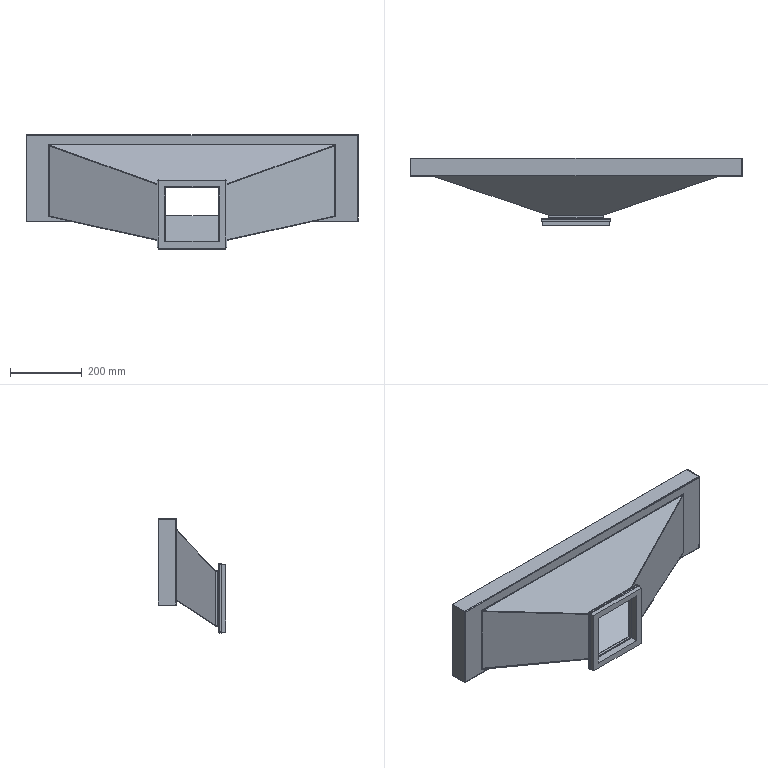Part | SolidWorks | 7 solids | 190 faces | box 927 x 189 x 319.6 mm | volume 886288 mm3 | plane 138 | cylinder 36 | spline 16 | commonest cylinder face diameters 2 x12 5 x8 0.1 x4 3.1 x4 4.4 x4 10 x4